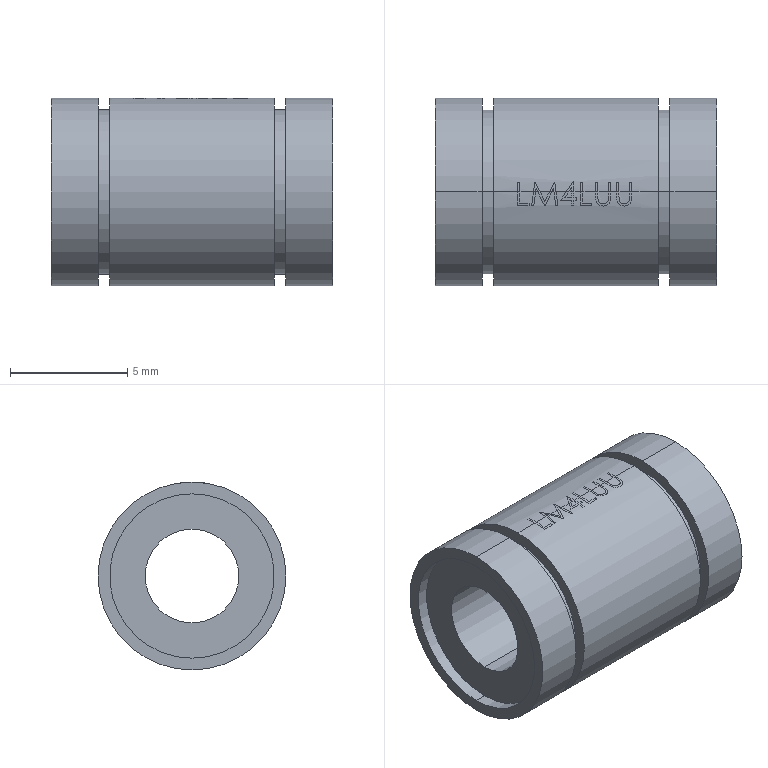Part | SolidWorks | features Emboss 1, Revolution 1 | 1 solid | 48 faces | box 12 x 8 x 8 mm | volume 414.691 mm3 | cylinder 40 | plane 8 | commonest cylinder face diameters 8 x30 7 x8 4 x2